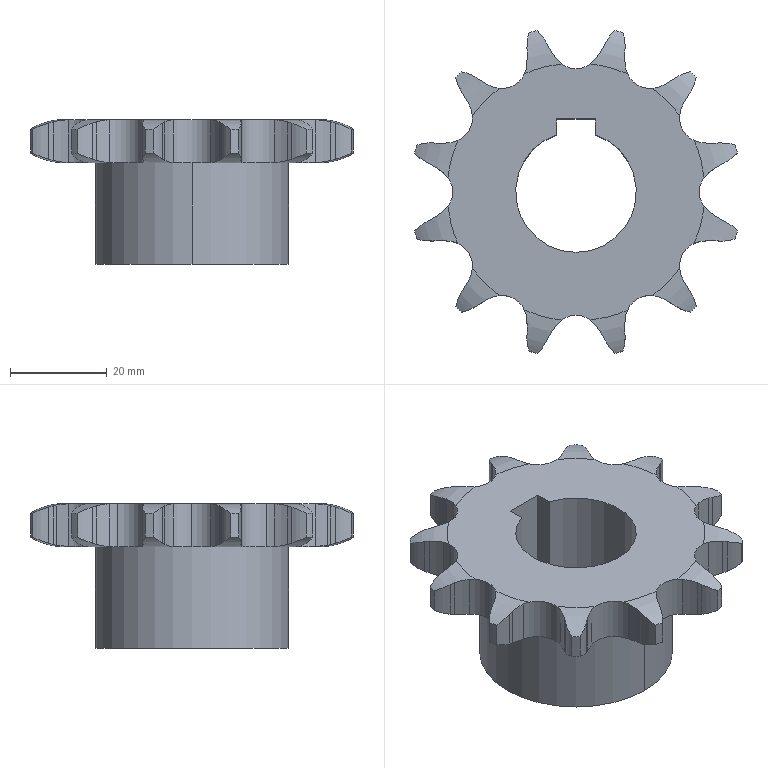Part | SolidWorks | features BaseBody 1 | 1 solid | 137 faces | box 66.851 x 66.851 x 30 mm | volume 34006 mm3 | cylinder 83 | plane 30 | spline 24 | commonest cylinder face diameters 17.16 x26 26.518 x26 10.262 x15 68.771 x12 25 x2 40 x2